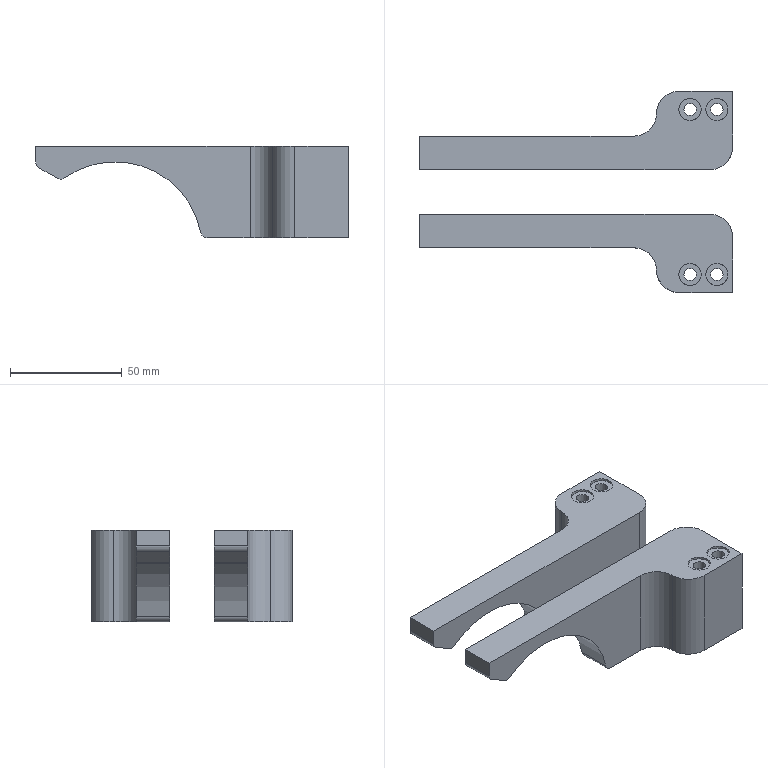NC program | NX | posted with a generic post | part box 140 x 90 x 41 mm
Lines 43 to 1050 of 29499:
(ADAPTIVE_MILLING_COPY , TOOL : D12C)
N72 T12 M6
N74 G54
N76 G17 G0 G90 X84.203 Y0.033 S9500 M3
N78 G43 Z30. H12
N80 Z-17.5
N82 G94 G1 Z-20.5 F1000.
N84 X82.519 Y0.626 F3000.
N86 G3 X81.036 Y0.033 R1.218
N88 X80.298 Y-3.273 R9.619
N90 X80.016 Y-14.066 R137.397
N92 G2 X79.975 Y-19.765 R266.591
N94 X76.756 Y-24.703 R7.183
N96 X70.601 Y-26.923 R14.584
N98 X61.923 Y-27.443 R65.22
N100 G1 X60.798 Y-27.455
N102 X59.598 Y-27.465
N104 X58.173 Y-27.473
N106 X56.223 Y-27.479
N108 X53.373 Y-27.484
N110 X48.198 Y-27.486
N112 X5.523
N114 X-71.727 Y-27.483
N116 X-71.876 Y-27.48
N118 X-71.951 Y-27.477
N120 X-72.101 Y-27.467
N122 X-72.176 Y-27.46
N124 G2 X-77.107 Y-24.364 R7.106
N126 X-79.409 Y-18.163 R14.366
N128 X-79.95 Y-8.812 R68.401
N130 G1 X-79.96 Y-7.687
N132 X-79.97 Y-6.262
N134 X-79.977 Y-4.537
N136 X-79.982 Y-2.137
N138 X-79.985 Y1.763
N140 X-79.987 Y12.113
N142 Y19.238
N144 X-79.983 Y19.388
N146 X-79.979 Y19.463
N148 X-79.969 Y19.613
N150 X-79.962 Y19.687
N152 G2 X-76.855 Y24.611 R7.108
N154 X-70.8 Y26.884 R14.2
N156 X-62.05 Y27.437 R61.812
N158 G1 X-61. Y27.45
N160 X-59.8 Y27.46
N162 X-58.225 Y27.469
N164 X-56.276 Y27.475
N166 X-53.501 Y27.48
N168 X-48.476 Y27.483
N170 X-15.026
N172 X71.674
N174 X71.824 Y27.481
N176 X71.899 Y27.479
N178 X71.974 Y27.475
N180 X72.124 Y27.465
N182 G2 X77.119 Y24.344 R7.087
N184 X79.424 Y18.065 R14.479
N186 X79.941 Y9.463 R64.779
N188 X79.907 Y2.64 R97.021
N190 G3 X79.041 Y-14.052 R135.629
N192 G2 X78.822 Y-17.712 R17.163
N194 X74.073 Y-23.799 R9.545
N196 X67.015 Y-25.945 R19.
N198 X56.757 Y-26.44 R91.333
N200 G1 X55.482 Y-26.45
N202 X53.907 Y-26.459
N204 X51.882 Y-26.466
N206 X49.033 Y-26.471
N208 X44.308 Y-26.474
N210 X28.333 Y-26.475
N212 X-68.343 Y-26.472
N214 X-68.492 Y-26.47
N216 X-68.717 Y-26.464
N218 X-68.867 Y-26.456
N220 G2 X-75.943 Y-22.109 R9.111
N222 X-78.354 Y-15.146 R17.399
N224 X-78.931 Y-5.045 R77.877
N226 G1 X-78.943 Y-3.92
N228 X-78.953 Y-2.57
N230 X-78.961 Y-0.92
N232 X-78.968 Y1.255
N234 X-78.972 Y4.33
N236 X-78.975 Y9.805
N238 G2 X-78.924 Y16.778 R130.078
N240 X-74.451 Y23.543 R9.204
N242 X-67.459 Y25.876 R17.79
N244 X-57.431 Y26.429 R79.927
N246 G1 X-56.231 Y26.441
N248 X-54.806 Y26.451
N250 X-53.082 Y26.459
N252 X-50.757 Y26.465
N254 X-47.307 Y26.469
N256 X-40.632 Y26.471
N258 X68.343 Y26.472
N260 X68.493 Y26.47
N262 X68.643 Y26.466
N264 X68.793 Y26.46
N266 X68.943 Y26.451
N268 G2 X75.904 Y22.17 R9.118
N270 X78.351 Y15.143 R17.3
N272 X78.591 Y0.177 R67.118
N274 G3 X78.048 Y-13.685 R225.078
N276 G2 X75.588 Y-20.034 R10.779
N278 X71.486 Y-23.506 R6.532
N280 X62.443 Y-25.167 R33.006
N282 X46.548 Y-25.458 R274.59
N284 G1 X42.423 Y-25.462
N286 X33.273 Y-25.463
N288 X-65.502 Y-25.46
N290 X-65.727 Y-25.458
N292 X-65.952 Y-25.452
N294 X-66.102 Y-25.447
N296 G2 X-74.971 Y-20.027 R10.513
N298 X-77.327 Y-12.644 R19.888
N300 X-77.914 Y-2.092 R86.472
N302 X-77.927 Y14.032 R598.657
N304 X-75.65 Y19.879 R10.74
N306 X-71.556 Y23.478 R6.436
N308 X-62.666 Y25.146 R32.567
N310 X-48.646 Y25.451 R229.068
N312 G1 X-45.796 Y25.456
N314 X-41.146 Y25.459
N316 X-28.396 Y25.46
N318 X65.504
N320 X65.729 Y25.457
N322 X65.954 Y25.452
N324 G2 X74.972 Y20.025 R10.525
N326 X77.326 Y12.641 R19.956
N328 X77.619 Y1.565 R54.742
N330 G3 X77.071 Y-11.773 R612.256
N332 G2 X76.164 Y-15.859 R15.904
N334 X75.972 Y-18.935 R17.38
N336 G1 X75.576 Y-20.068
N338 G3 X76.15 Y-17.465 R7.23
N340 G1 Y-15.989
N342 X76.502 Y-10.076
N344 X76.549 Y-8.801
N346 X76.576 Y-8.052
N348 X76.677 Y-5.504
N350 X76.808 Y-2.582
N352 X76.874 Y-1.308
N354 X76.897 Y-0.859
N356 X77.019 Y1.688
N358 X77.053 Y2.512
N360 X77.081 Y3.262
N362 G3 X76.36 Y14.012 R45.331
N364 X73.299 Y20.691 R14.854
N366 X66.922 Y24.215 R11.109
N368 X59.457 Y24.812 R41.057
N370 G1 X58.632 Y24.823
N372 X57.657 Y24.833
N374 X56.382 Y24.841
N376 X54.657 Y24.847
N378 X52.257 Y24.851
N380 X47.382 Y24.854
N382 X-47.043
N384 X-52.068 Y24.832
N386 G3 X-64.129 Y24.36 R127.574
N388 X-68.434 Y23.65 R45.283
N390 X-71.435 Y23.472 R14.718
N392 G1 X-72.601 Y23.064
N394 G2 X-69.965 Y23.65 R7.29
N396 G1 X-68.434
N398 G3 X-53.886 Y23.787 R352.72
N400 G2 X-34.836 Y23.853 R978.866
N402 G1 X-33.936 Y23.852
N404 X-33.111 Y23.853
N406 X-32.061 Y23.852
N408 X-31.311 Y23.854
N410 X-30.111 Y23.852
N412 X-29.361 Y23.854
N414 X-28.236 Y23.852
N416 X-27.261 Y23.854
N418 X-26.586 Y23.853
N420 X-25.311 Y23.855
N422 X-24.336 Y23.853
N424 X-23.586 Y23.854
N426 X-22.536 Y23.853
N428 X-21.786 Y23.854
N430 X-20.586 Y23.853
N432 X-19.836 Y23.854
N434 X-18.561 Y23.852
N436 X-17.661 Y23.855
N438 X-16.911 Y23.854
N440 X-15.636 Y23.855
N442 X-15.186 Y23.856
N444 X-14.286 Y23.854
N446 X-13.386 Y23.855
N448 X-12.561 Y23.854
N450 X-11.586 Y23.855
N452 X-10.686 Y23.853
N454 X-9.636 Y23.856
N456 X-8.661 Y23.853
N458 X-7.611 Y23.856
N460 X-6.786 Y23.854
N462 X-5.586 Y23.855
N464 X-4.911 Y23.854
N466 X-3.786 Y23.856
N468 X-2.661 Y23.854
N470 X-1.536 Y23.856
N472 X-0.786 Y23.854
N474 X0.414 Y23.856
N476 X1.389 Y23.853
N478 X2.364 Y23.855
N480 X3.339 Y23.853
N482 X4.389 Y23.855
N484 X5.214 Y23.854
N486 X6.414 Y23.855
N488 X7.089 Y23.854
N490 X8.139 Y23.855
N492 X8.589 Y23.856
N494 X9.264 Y23.855
N496 X10.539 Y23.856
N498 X11.439 Y23.854
N500 X12.489 Y23.856
N502 X13.464 Y23.854
N504 X14.289 Y23.855
N506 X15.414 Y23.853
N508 X16.314 Y23.855
N510 X17.064 Y23.854
N512 X18.339 Y23.855
N514 X19.314 Y23.853
N516 X20.364 Y23.855
N518 X21.264 Y23.854
N520 X22.164 Y23.855
N522 X23.064 Y23.853
N524 X24.114 Y23.855
N526 X24.939 Y23.854
N528 X25.989 Y23.855
N530 X26.664 Y23.854
N532 X27.714 Y23.855
N534 X28.089 Y23.856
N536 X28.989 Y23.854
N538 X29.739
N540 X31.014 Y23.853
N542 X31.464 Y23.852
N544 X32.364 Y23.854
N546 X33.264 Y23.853
N548 X34.164 Y23.854
N550 X35.214 Y23.853
N552 X36.039 Y23.854
N554 X37.014 Y23.853
N556 X37.764 Y23.854
N558 X38.814 Y23.853
N560 X39.789 Y23.855
N562 X40.464 Y23.854
N564 X41.439 Y23.855
N566 X41.889
N568 X42.789 Y23.853
N570 X43.539 Y23.854
N572 X44.814 Y23.852
N574 X45.339
N576 G2 X61.462 Y23.707 R414.659
N578 X67.562 Y22.615 R19.204
N580 X73.963 Y16.194 R11.998
N582 X74.914 Y13.565 R24.795
N584 G1 X75.341 Y12.536
N586 X75.371 Y12.442
N588 X75.94 Y10.075
N590 X75.955 Y9.977
N592 X76.148 Y7.525
N594 X76.15 Y7.475
N596 Y-15.7
N598 G3 X78.17 Y-16.576 R1.201
N600 X78.555 Y-15.902 Z-20.467 R1.571
N602 G1 X79.119 Y-14.389 Z-20.4
N604 X79.935 Y-12.171
N606 X79.968 Y-11.881
N608 X79.842 Y3.737
N610 G3 X79.591 Y10.865 R164.822
N612 X78.585 Y12.002 R1.247
N614 G1 X76.287 Y12.692 Z-20.5
N616 X75.512 Y12.939
N618 G2 X74.914 Y13.565 R1.232
N620 G1 X74.409 Y14.786
N622 X74.364 Y14.874
N624 G3 X72.66 Y17.5 R21.63
N626 X70.266 Y19.905 R13.845
N628 G1 X69.53 Y20.533
N630 X69.45 Y20.592
N632 X67.374 Y21.864
N634 X67.286 Y21.909
N636 X65.036 Y22.841
N638 X64.942 Y22.871
N640 X62.575 Y23.44
N642 X62.477 Y23.455
N644 X60.025 Y23.648
N646 X59.975 Y23.65
N648 X-58.975
N650 G2 X-59.808 Y25.714 R1.201
N652 X-59.169 Y26.058 Z-20.47 R1.662
N654 G1 X-57.606 Y26.639 Z-20.4
N656 X-55.438 Y27.435
N658 X-55.156 Y27.468
N660 X57.496
N662 G2 X66.055 Y26.387 R34.687
N664 G1 X70.266 Y25.305
N666 G2 X71.051 Y23.628 R1.204
N668 G1 X70.883 Y23.274
N670 X69.913 Y21.217 Z-20.495
N672 X69.878 Y21.097 Z-20.5
N674 G3 X70.266 Y19.905 R1.212
N676 G1 X71.382 Y18.952
N678 X71.452 Y18.882
N680 X73.033 Y17.03
N682 G3 X73.926 Y16.61 R1.227
N684 G1 X74.444 Y16.601
N686 X76.844 Y16.562 Z-20.4
N688 G2 X77.67 Y16.404 R1.591
N690 X78.249 Y15.633 R1.228
N692 G1 X79.148 Y11.747
N694 G2 X79.781 Y6.816 R34.643
N696 G1 X81.012 Y-15.945
N698 G2 X79.58 Y-20.859 R7.765
N700 G1 X78.001 Y-23.064
N702 G2 X76.841 Y-23.552 R1.212
N704 G1 X74.467 Y-23.201 Z-20.5
N706 X73.725 Y-23.085
N708 X72.981 Y-22.997
N710 X72.789 Y-23.019
N712 X72.601 Y-23.064
N714 G2 X69.065 Y-23.657 R7.864
N716 X49.062 Y-24.433 R219.712
N718 G1 X46.812 Y-24.441
N720 X43.962 Y-24.446
N722 X39.612 Y-24.45
N724 X30.237 Y-24.452
N726 X-62.913 Y-24.449
N728 X-63.288 Y-24.446
N730 G2 X-74.046 Y-18.065 R11.668
N732 X-76.335 Y-10.265 R22.381
N734 X-76.9 Y0.515 R96.407
N736 X-76.906 Y11.839 R322.039
N738 X-76.158 Y15.578 R16.045
N740 X-75.972 Y18.935 R18.068
N742 G1 X-75.601 Y19.997
N744 G3 X-76.15 Y17.465 R7.108
N746 G1 Y15.653
N748 G3 X-76.05 Y-6.389 R251.537
N750 X-74.556 Y-14.857 R32.177
N752 X-69.766 Y-21.394 R12.725
N754 X-63.494 Y-23.49 R14.158
N756 X-54.881 Y-23.829 R81.129
N758 G1 X-53.381 Y-23.835
N760 X-51.131 Y-23.84
N762 X-47.081 Y-23.843
N764 X-2.981 Y-23.845
N766 X44.644 Y-23.846
N768 G3 X59.456 Y-23.65 R522.335
N770 G1 X69.281
N772 X46.025
N774 X45.975 Y-23.648
N776 G2 X41.797 Y-23.181 R36.671
N778 G3 X32.431 Y-22.873 R101.962
N780 G1 X30.631 Y-22.866
N782 X28.081 Y-22.861
N784 X23.881 Y-22.858
N786 X9.931 Y-22.856
N788 X-15.494
N790 X-17.069 Y-22.849
N792 X-18.269 Y-22.85
N794 X-19.019 Y-22.848
N796 X-19.844
N798 X-20.294
N800 X-21.119 Y-22.846
N802 X-22.394 Y-22.847
N804 X-23.294 Y-22.845
N806 X-24.344 Y-22.846
N808 X-25.094 Y-22.845
N810 X-26.144 Y-22.846
N812 X-27.119 Y-22.843
N814 X-28.169 Y-22.845
N816 X-28.994 Y-22.844
N818 X-30.119 Y-22.845
N820 X-30.869 Y-22.844
N822 X-31.919 Y-22.845
N824 X-32.894 Y-22.843
N826 X-33.569 Y-22.844
N828 X-34.544 Y-22.843
N830 X-34.994 Y-22.842
N832 X-35.894 Y-22.844
N834 X-36.644 Y-22.843
N836 X-37.919 Y-22.845
N838 X-38.294
N840 X-38.969 Y-22.844
N842 X-40.169 Y-22.845
N844 X-40.619 Y-22.846
N846 X-41.519 Y-22.843
N848 X-42.569 Y-22.845
N850 X-43.394 Y-22.843
N852 X-44.519 Y-22.845
N854 X-45.344 Y-22.843
N856 X-46.394 Y-22.844
N858 X-47.069 Y-22.843
N860 X-48.344
N862 X-49.469 Y-22.84
N864 G2 X-60.94 Y-22.621 R180.414
N866 X-67.415 Y-20.914 R15.593
N868 X-73.137 Y-14.1 R13.277
N870 X-74.934 Y-5.544 R29.569
N872 G1 X-74.971 Y-5.096
N874 X-75.005 Y-4.647
N876 X-75.03 Y-4.273
N878 X-75.068 Y-3.674
N880 X-75.097 Y-3.15
N882 X-75.127 Y-2.551
N884 X-75.156 Y-1.876
N886 X-75.182 Y-1.202
N888 X-75.187 Y-1.052
N890 X-75.192 Y-0.977
N892 X-75.202 Y-0.903
N894 X-75.216 Y-0.829
N896 G3 X-75.564 Y-0.101 R4.399
N898 G2 X-76.15 Y2.535 R7.211
N900 G1 Y15.135
N902 X-76.146 Y2.465
N904 G3 X-75.564 Y-0.101 R7.131
N906 G1 X-75.346 Y-0.479
N908 G2 X-74.773 Y-2.484 R5.321
N910 G3 X-73.709 Y-9.602 R115.381
N912 X-70.623 Y-16.774 R17.487
N914 X-62.946 Y-21.399 R13.075
N916 X-54.821 Y-22.167 R41.287
N918 X-33.672 Y-22.243 R989.782
N920 G1 X-32.322 Y-22.246
N922 X-31.272 Y-22.244
N924 X-30.822 Y-22.245
N926 X-29.772 Y-22.243
N928 X-28.797 Y-22.245
N930 X-27.372 Y-22.243
N932 X-26.922 Y-22.244
N934 X-26.022 Y-22.243
N936 X-24.522 Y-22.246
N938 X-24.072
N940 X-22.347 Y-22.249
N942 X-21.672 Y-22.247
N944 X-20.697 Y-22.249
N946 X-18.222 Y-22.252
N948 X-17.022 Y-22.251
N950 X-16.572 Y-22.253
N952 X-14.697 Y-22.251
N954 X-14.247 Y-22.253
N956 X-12.447 Y-22.252
N958 X-11.997 Y-22.253
N960 X-10.122 Y-22.252
N962 X-9.672 Y-22.253
N964 X-7.797 Y-22.252
N966 X-7.347 Y-22.253
N968 X-5.547 Y-22.252
N970 X-5.097 Y-22.253
N972 X-3.222 Y-22.252
N974 X-2.772 Y-22.253
N976 X-0.972 Y-22.252
N978 X-0.522 Y-22.253
N980 X1.353 Y-22.252
N982 X1.803 Y-22.253
N984 X3.603 Y-22.252
N986 X4.053 Y-22.254
N988 X5.928 Y-22.252
N990 X6.378 Y-22.254
N992 X8.178 Y-22.252
N994 X8.628 Y-22.254
N996 X10.428 Y-22.252
N998 X10.878 Y-22.254
N1000 X12.678 Y-22.252
N1002 X13.128 Y-22.254
N1004 X14.853 Y-22.252
N1006 X15.303 Y-22.254
N1008 X16.953 Y-22.253
N1010 X17.403 Y-22.254
N1012 X18.978 Y-22.253
N1014 X19.428 Y-22.255
N1016 G2 X38.402 Y-22.39 R667.407
N1018 X40.24 Y-22.541 R11.704
N1020 G1 X40.964 Y-22.841
N1022 X41.058 Y-22.871
N1024 X43.318 Y-23.414
N1026 X41.058 Y-22.871
N1028 X40.964 Y-22.841
N1030 X40.24 Y-22.541
N1032 G3 X36.023 Y-21.575 R12.205
N1034 X24.105 Y-21.275 R159.746
N1036 G1 X23.58 Y-21.271
N1038 X22.38 Y-21.265
N1040 X21.18 Y-21.264
N1042 X20.58 Y-21.263
N1044 X19.83 Y-21.26
N1046 X19.005 Y-21.259
N1048 X18.405 Y-21.26
N1050 X17.655 Y-21.257
N1052 X16.53
N1054 X16.005 Y-21.258
N1056 X15.405 Y-21.256
N1058 X14.13
N1060 X13.68
N1062 X12.855 Y-21.254
N1064 X11.88 Y-21.255
N1066 X10.98 Y-21.253
N1068 X9.705 Y-21.255
N1070 X8.955 Y-21.254
N1072 X8.055
N1074 X7.605 Y-21.255
N1076 X6.555 Y-21.252
N1078 X5.73 Y-21.254
N1080 X4.755 Y-21.252
N1082 X4.23
N1084 X3.405 Y-21.254
N1086 X2.28 Y-21.251
N1088 X1.305 Y-21.254
N1090 X0.03 Y-21.251
N1092 X-0.645 Y-21.252
N1094 X-1.92 Y-21.251
N1096 X-2.52 Y-21.25
N1098 X-3.195 Y-21.251
N1100 X-4.32 Y-21.25
N1102 X-4.77
N1104 X-5.67 Y-21.252
N1106 X-6.42 Y-21.251
N1108 X-7.47 Y-21.253
N1110 X-8.22 Y-21.251
N1112 X-9.12 Y-21.253
N1114 X-9.945 Y-21.251
N1116 X-11.145 Y-21.253
N1118 X-12.045 Y-21.252
N1120 X-13.17 Y-21.254
N1122 X-13.92 Y-21.252
N1124 X-15.12 Y-21.253
N1126 X-15.87 Y-21.252
N1128 X-16.92 Y-21.253
N1130 X-18.12 Y-21.249
N1132 X-19.245 Y-21.251
N1134 X-20.37 Y-21.248
N1136 X-21.345 Y-21.25
N1138 X-22.62 Y-21.245
N1140 X-23.745 Y-21.247
N1142 X-24.645 Y-21.245
N1144 X-25.695 Y-21.246
N1146 X-26.595 Y-21.244
N1148 X-27.795 Y-21.246
N1150 X-28.545 Y-21.245
N1152 X-29.67 Y-21.246
N1154 X-30.795 Y-21.245
N1156 X-31.77
N1158 X-32.67 Y-21.243
N1160 X-33.57 Y-21.244
N1162 X-34.545 Y-21.242
N1164 X-35.445 Y-21.244
N1166 X-36.495 Y-21.242
N1168 X-37.47 Y-21.244
N1170 X-38.52 Y-21.242
N1172 X-39.195 Y-21.243
N1174 X-40.245 Y-21.242
N1176 X-40.845 Y-21.241
N1178 X-41.52 Y-21.242
N1180 X-42.495 Y-21.24
N1182 X-42.87 Y-21.239
N1184 X-43.545
N1186 X-44.595 Y-21.236
N1188 X-45.12
N1190 X-45.645
N1192 G2 X-57.79 Y-20.982 R195.106
N1194 X-64.628 Y-19.427 R20.046
N1196 X-71.238 Y-12.455 R13.483
N1198 X-73.137 Y-5.761 R29.243
N1200 G3 X-73.859 Y-2.391 R33.185
N1202 X-74.846 Y-1.274 R6.606
N1204 G1 X-75.285 Y-0.576
N1206 X-74.846 Y-1.274
N1208 X-74.758 Y-1.385
N1210 X-74.064 Y-2.079
N1212 G2 X-73.24 Y-3.658 R3.699
N1214 X-71.754 Y-9.004 R754.546
N1216 G3 X-67.846 Y-15.921 R16.493
N1218 X-60.27 Y-19.783 R14.868
N1220 X-52.142 Y-20.543 R45.399
N1222 X-30.768 Y-20.644 R964.708
N1224 G1 X-30.093 Y-20.645
N1226 X-29.568
N1228 X-25.968 Y-20.649
N1230 X-22.368 Y-20.65
N1232 X-20.043 Y-20.648
N1234 X-18.618
N1236 X-17.943 Y-20.65
N1238 X-16.068 Y-20.649
N1240 X-15.468 Y-20.65
N1242 X-14.418 Y-20.649
N1244 X-13.968 Y-20.65
N1246 X-8.493 Y-20.648
N1248 X-3.018 Y-20.649
N1250 X2.457 Y-20.655
N1252 X3.357 Y-20.656
N1254 X4.257 Y-20.654
N1256 X5.232 Y-20.656
N1258 X5.682 Y-20.655
N1260 X6.432 Y-20.656
N1262 X6.882
N1264 X7.332
N1266 X7.932 Y-20.655
N1268 X8.457
N1270 X8.682
N1272 X9.282 Y-20.656
N1274 X10.407 Y-20.654
N1276 X11.232 Y-20.656
N1278 X11.757
N1280 X15.357 Y-20.661
N1282 X18.957 Y-20.662
N1284 G2 X33.954 Y-20.87 R347.657
N1286 X37.743 Y-21.334 R18.383
N1288 G1 X37.811 Y-21.365
N1290 G2 X38.352 Y-22.668 R1.208
N1292 X37.62 Y-23.513 Z-20.452 R1.245
N1294 G1 X36.511 Y-24.067 Z-20.4
N1296 X34.529 Y-25.057
N1298 X34.268 Y-25.148
N1300 X33.993 Y-25.184
N1302 X-43.257
N1304 G2 X-56.665 Y-24.074 R82.222
N1306 G1 X-59.254 Y-23.647
N1308 X-61.838 Y-23.197
N1310 G2 X-67.156 Y-21.265 R21.108
N1312 X-70.794 Y-18.213 R12.698
N1314 X-73.676 Y-13.871 R20.746
N1316 X-75.482 Y-9.76 R61.41
N1318 G1 X-76.605 Y-6.914
N1320 G2 X-76.661 Y-6.22 R1.251
N1322 G1 X-76.219 Y-4.181
N1324 X-75.896 Y-2.734 Z-20.462
N1326 G2 X-75.336 Y-2.037 Z-20.5 R1.202
N1328 X-73.905 Y-2.238 R1.208
N1330 X-72.71 Y-4.239 R5.025
N1332 G3 X-70.867 Y-9.552 R389.797
N1334 X-60.789 Y-18.728 R14.651
N1336 X-52.111 Y-19.881 R36.875
N1338 X-31.188 Y-20.043 R698.71
N1340 G1 X-30.288 Y-20.046
N1342 X-29.538 Y-20.045
N1344 X-28.863 Y-20.047
N1346 X-27.963 Y-20.046
N1348 X-27.438 Y-20.048
N1350 X-26.163 Y-20.046
N1352 X-25.713 Y-20.048
N1354 X-22.713 Y-20.044
N1356 X-22.113 Y-20.046
N1358 X-20.988 Y-20.045
N1360 X-20.463 Y-20.046
N1362 X-19.413 Y-20.045
N1364 X-19.038 Y-20.047
N1366 X-18.363 Y-20.046
N1368 X-17.838 Y-20.047
N1370 X-17.013 Y-20.046
N1372 X-15.513 Y-20.045
N1374 X-15.138 Y-20.047
N1376 X-12.288 Y-20.044
N1378 X-11.838 Y-20.046
N1380 X-10.038 Y-20.044
N1382 X-9.513 Y-20.046
N1384 X-8.088 Y-20.044
N1386 X-7.563 Y-20.046
N1388 X-6.438 Y-20.045
N1390 X-5.913 Y-20.047
N1392 X-5.013 Y-20.046
N1394 X-4.413 Y-20.048
N1396 X-3.513 Y-20.047
N1398 X-2.838 Y-20.049
N1400 X-2.013
N1402 X-1.263 Y-20.051
N1404 X-0.513 Y-20.05
N1406 X0.312 Y-20.053
N1408 X2.337 Y-20.051
N1410 X2.937 Y-20.053
N1412 X3.387
N1414 X3.912 Y-20.054
N1416 X4.362
N1418 X4.812 Y-20.055
N1420 X5.412 Y-20.054
N1422 X6.387 Y-20.056
N1424 X7.962 Y-20.053
N1426 X10.287 Y-20.052
N1428 X12.312 Y-20.055
N1430 X13.437 Y-20.059
N1432 X14.562 Y-20.058
N1434 X15.087 Y-20.06
N1436 G2 X33.159 Y-20.262 R435.476
N1438 X36.583 Y-20.635 R21.05
N1440 G1 X36.653 Y-20.664
N1442 X36.721 Y-20.696
N1444 X38.626 Y-21.864
N1446 X38.714 Y-21.909
N1448 X39.545 Y-22.253
N1450 X38.714 Y-21.909
N1452 X38.626 Y-21.864
N1454 X36.721 Y-20.696
N1456 G3 X33.619 Y-19.654 R7.433
N1458 X24.942 Y-19.132 R65.219
N1460 X4.917 Y-19.056 R998.037
N1462 G1 X4.242 Y-19.057
N1464 X3.417 Y-19.055
N1466 X1.992 Y-19.056
N1468 X1.017 Y-19.053
N1470 X0.117
N1472 X-0.933 Y-19.05
N1474 X-1.608
N1476 X-2.883 Y-19.047
N1478 X-3.258 Y-19.046
N1480 X-4.233 Y-19.048
N1482 X-5.208 Y-19.046
N1484 X-6.333 Y-19.047
N1486 X-7.158 Y-19.046
N1488 X-8.358 Y-19.047
N1490 X-9.333 Y-19.044
N1492 X-10.383 Y-19.047
N1494 X-11.208 Y-19.045
N1496 X-12.183 Y-19.047
N1498 X-13.158 Y-19.045
N1500 X-13.833 Y-19.046
N1502 X-14.883 Y-19.045
N1504 X-15.408
N1506 X-16.008 Y-19.046
N1508 X-16.983 Y-19.045
N1510 X-17.733 Y-19.046
N1512 X-18.858 Y-19.044
N1514 X-19.458 Y-19.045
N1516 X-20.583 Y-19.044
N1518 X-21.332 Y-19.046
N1520 X-22.457 Y-19.045
N1522 X-23.057 Y-19.046
N1524 X-23.957 Y-19.045
N1526 X-24.707 Y-19.044
N1528 X-25.607 Y-19.046
N1530 X-26.732 Y-19.044
N1532 X-27.482 Y-19.046
N1534 X-28.532 Y-19.044
N1536 X-29.282 Y-19.045
N1538 X-30.332 Y-19.043
N1540 X-31.157 Y-19.044
N1542 X-32.132 Y-19.041
N1544 X-33.182 Y-19.042
N1546 X-34.157 Y-19.039
N1548 X-35.432 Y-19.042
N1550 X-36.857 Y-19.037
N1552 X-37.457 Y-19.038
N1554 X-39.182 Y-19.034
N1556 X-40.907 Y-19.027
N1558 X-42.782 Y-19.016
N1560 G2 X-54.549 Y-18.662 R149.256
N1562 X-62.366 Y-16.717 R22.553
N1564 X-69.1 Y-9.905 R15.054
N1566 X-71.479 Y-4.644 R130.122
N1568 G3 X-72.388 Y-3.194 R4.304
N1570 G1 X-72.449 Y-3.15
N1572 X-72.512 Y-3.11
N1574 X-72.577 Y-3.073
N1576 X-72.601 Y-3.064
N1578 X-72.728 Y-3.003
N1580 X-73.774 Y-2.346
N1582 X-73.833 Y-2.299
N1584 X-72.728 Y-3.003
N1586 X-72.577 Y-3.073
N1588 G2 X-71.461 Y-4.144 R2.481
N1590 X-69.189 Y-8.369 R50.2
N1592 G3 X-63.783 Y-14.78 R17.102
N1594 X-55.83 Y-17.723 R19.303
N1596 X-46.109 Y-18.363 R69.952
N1598 X-25.86 Y-18.444 R986.729
N1600 G1 X-24.06 Y-18.442
N1602 X-23.685 Y-18.443
N1604 X-22.935 Y-18.442
N1606 X-22.485 Y-18.443
N1608 X-21.735 Y-18.444
N1610 X-21.21 Y-18.443
N1612 X-20.76 Y-18.444
N1614 X-19.185 Y-18.442
N1616 X-18.36 Y-18.444
N1618 X-17.535 Y-18.443
N1620 X-17.085 Y-18.444
N1622 X-15.36 Y-18.442
N1624 X-14.46 Y-18.444
N1626 X-13.935
N1628 X-12.735 Y-18.446
N1630 X-12.135 Y-18.445
N1632 X-10.41 Y-18.448
N1634 X-9.51 Y-18.446
N1636 X-8.685 Y-18.448
N1638 X-8.16 Y-18.446
N1640 X-6.36 Y-18.449
N1642 X-5.835
N1644 X-3.885 Y-18.452
N1646 X-1.635 Y-18.455
N1648 X-1.185 Y-18.454
N1650 X-0.51 Y-18.456
N1652 X1.14 Y-18.453
N1654 X1.815 Y-18.455
N1656 X2.49 Y-18.454
N1658 X2.94 Y-18.455
N1660 X3.54 Y-18.454
N1662 X4.815 Y-18.457
N1664 G2 X27.539 Y-18.609 R916.601
N1666 X34.245 Y-19.286 R36.704
N1668 X35.529 Y-19.73 R4.915
N1670 G1 X36.47 Y-20.533
N1672 X35.529 Y-19.73
N1674 G3 X32.78 Y-18.431 R5.998
N1676 X25.71 Y-17.647 R36.82
N1678 X4.187 Y-17.461 R753.21
N1680 G1 X2.837 Y-17.459
N1682 X1.487 Y-17.46
N1684 X0.587 Y-17.457
N1686 X-0.538
N1688 X-1.588 Y-17.454
N1690 X-2.488
N1692 X-3.688 Y-17.45
N1694 X-4.513 Y-17.451
N1696 X-5.488 Y-17.449
N1698 X-6.238 Y-17.45
N1700 X-7.138 Y-17.448
N1702 X-8.113 Y-17.449
N1704 X-8.863 Y-17.447
N1706 X-10.063 Y-17.448
N1708 X-10.963 Y-17.446
N1710 X-11.863
N1712 X-12.763 Y-17.445
N1714 X-13.888 Y-17.446
N1716 X-14.788 Y-17.444
N1718 X-15.838 Y-17.445
N1720 X-16.663 Y-17.443
N1722 X-17.713 Y-17.445
N1724 X-18.688 Y-17.443
N1726 X-19.513 Y-17.444
N1728 X-20.413 Y-17.443
N1730 X-21.613 Y-17.445
N1732 X-22.288 Y-17.444
N1734 X-23.413 Y-17.445
N1736 X-23.938
N1738 X-24.613 Y-17.444
N1740 X-25.888 Y-17.445
N1742 X-26.938 Y-17.442
N1744 X-27.688 Y-17.443
N1746 X-28.813 Y-17.441
N1748 X-29.563 Y-17.439
N1750 G2 X-48.836 Y-17.26 R602.891
N1752 X-57.303 Y-16.205 R39.528
N1754 X-67.118 Y-9.146 R16.606
N1756 G3 X-70.057 Y-4.617 R307.957
N1758 X-71.173 Y-3.539 R2.814
N1760 G1 X-71.244 Y-3.515
N1762 X-71.261 Y-3.508
N1764 X-71.298 Y-3.504
N1766 X-71.435 Y-3.472
N1768 X-72.568 Y-3.076
N1770 X-71.435 Y-3.472
N1772 X-71.298 Y-3.504
N1774 X-71.261 Y-3.508
N1776 G2 X-70.074 Y-4.244 R2.135
N1778 X-67.332 Y-7.806 R31.148
N1780 G3 X-61.192 Y-13.654 R19.464
N1782 X-52.938 Y-16.222 R22.297
N1784 X-42.384 Y-16.779 R93.146
N1786 X-23.934 Y-16.844 R989.622
N1788 G1 X-23.334 Y-16.843
N1790 X-22.134 Y-16.845
N1792 X-21.009 Y-16.843
N1794 X-19.959 Y-16.845
N1796 X-18.909 Y-16.843
N1798 X-18.384 Y-16.845
N1800 X-17.709 Y-16.843
N1802 X-16.284 Y-16.846
N1804 X-15.159 Y-16.844
N1806 X-14.634 Y-16.845
N1808 X-13.284 Y-16.843
N1810 X-12.834 Y-16.844
N1812 X-10.884 Y-16.843
N1814 X-10.284 Y-16.845
N1816 X-9.609 Y-16.844
N1818 X-8.634 Y-16.848
N1820 X-7.659 Y-16.846
N1822 X-6.759 Y-16.849
N1824 X-6.309
N1826 X-5.259 Y-16.852
N1828 X-3.909 Y-16.851
N1830 X-3.234 Y-16.853
N1832 X-1.584
N1834 X-1.134 Y-16.854
N1836 X0.216
N1838 X0.666 Y-16.856
N1840 X1.266 Y-16.855
N1842 X2.616 Y-16.861
N1844 X4.116 Y-16.86
N1846 X5.241 Y-16.865
N1848 X7.191
N1850 X7.716 Y-16.868
N1852 X8.691
N1854 X9.366 Y-16.871
N1856 G2 X26.538 Y-17.113 R406.931
N1858 X33.058 Y-18.035 R28.793
N1860 X34.307 Y-18.6 R3.498
N1862 G3 X35.188 Y-19.439 R7.393
N1864 G1 X34.618 Y-18.952
N1866 X34.548 Y-18.882
N1868 X34.307 Y-18.6
N1870 G3 X32.022 Y-17.233 R4.715
N1872 X25.374 Y-16.177 R27.164
N1874 X10.003 Y-15.884 R305.412
N1876 G1 X8.728 Y-15.878
N1878 X7.453 Y-15.875
N1880 X6.853 Y-15.871
N1882 X5.803 Y-15.869
N1884 X5.278
N1886 X4.528 Y-15.866
N1888 X3.328 Y-15.864
N1890 X2.803 Y-15.863
N1892 X2.128 Y-15.86
N1894 X1.228
N1896 X0.853
N1898 X0.103 Y-15.857
N1900 X-0.797 Y-15.858
N1902 X-1.847 Y-15.859
N1904 X-2.822 Y-15.854
N1906 X-3.722 Y-15.855
N1908 X-4.772 Y-15.851
N1910 X-5.822 Y-15.852
N1912 X-6.572 Y-15.849
N1914 X-7.472
N1916 X-8.072
N1918 X-8.822 Y-15.847
N1920 X-9.947 Y-15.848
N1922 X-10.772 Y-15.845
N1924 X-11.747 Y-15.846
N1926 X-12.722 Y-15.844
N1928 X-13.472 Y-15.846
N1930 X-14.672 Y-15.844
N1932 X-15.497 Y-15.845
N1934 X-16.322 Y-15.844
N1936 X-17.447 Y-15.846
N1938 X-18.197 Y-15.844
N1940 X-19.322 Y-15.845
N1942 X-20.222 Y-15.844
N1944 X-21.197 Y-15.845
N1946 X-22.322 Y-15.842
N1948 X-23.222 Y-15.843
N1950 X-24.347 Y-15.841
N1952 X-25.172 Y-15.842
N1954 X-26.072 Y-15.84
N1956 X-26.447 Y-15.839
N1958 G2 X-46.919 Y-15.637 R607.655
N1960 X-55.532 Y-14.535 R40.864
N1962 X-65.095 Y-8.518 R18.886
N1964 G3 X-68.558 Y-4.575 R99.861
N1966 X-69.827 Y-3.674 R3.139
N1968 G1 X-69.9 Y-3.658
N1970 X-69.932 Y-3.65
N1972 X-69.965
N1974 X-70.035 Y-3.646
N1976 X-71.228 Y-3.512
N1978 X-70.035 Y-3.646
N1980 X-69.965 Y-3.65
N1982 X-69.932
N1984 G2 X-68.462 Y-4.333 R2.566
N1986 X-65.047 Y-7.699 R36.791
N1988 G3 X-52.516 Y-14.372 R21.189
N1990 X-42.204 Y-15.137 R70.588
N1992 X-21.13 Y-15.243 R947.691
N1994 G1 X-19.855 Y-15.246
N1996 X-19.33 Y-15.245
N1998 X-17.83 Y-15.247
N2000 X-17.005 Y-15.245
N2002 X-16.48 Y-15.246
N2004 X-15.955 Y-15.245
N2006 X-15.655 Y-15.246
N2008 X-14.905 Y-15.244
N2010 X-13.855 Y-15.246
N2012 X-13.03 Y-15.245
N2014 X-12.28 Y-15.247
N2016 X-11.83 Y-15.246
N2018 X-10.03 Y-15.25
N2020 X-9.355 Y-15.248
N2022 X-8.23 Y-15.251
N2024 X-7.705 Y-15.252
N2026 X-7.48
N2028 X-7.105 Y-15.251
N2030 X-6.055 Y-15.254
N2032 X-5.605 Y-15.253
N2034 X-4.93 Y-15.254
N2036 X-4.255 Y-15.256
N2038 X-3.43 Y-15.255
N2040 X-3.055 Y-15.256
N2042 X-2.305 Y-15.255
N2044 X-1.48 Y-15.257
N2046 X-1.03
N2048 X-0.055
N2050 X0.47 Y-15.259
N2052 X0.92 Y-15.26
N2054 X3.32 Y-15.268
N2056 X3.995 Y-15.267
N2058 X4.82 Y-15.268
N2060 X5.27 Y-15.269
N2062 X5.87 Y-15.27
N2064 X6.695 Y-15.271
N2066 X7.52 Y-15.276
N2068 X7.745 Y-15.277
N2070 X8.495 Y-15.281
N2072 X9.395 Y-15.286
N2074 X9.92 Y-15.287
N2076 G2 X25.364 Y-15.612 R272.68
N2078 X31.854 Y-16.71 R26.007
N2080 X33.319 Y-17.443 R4.41